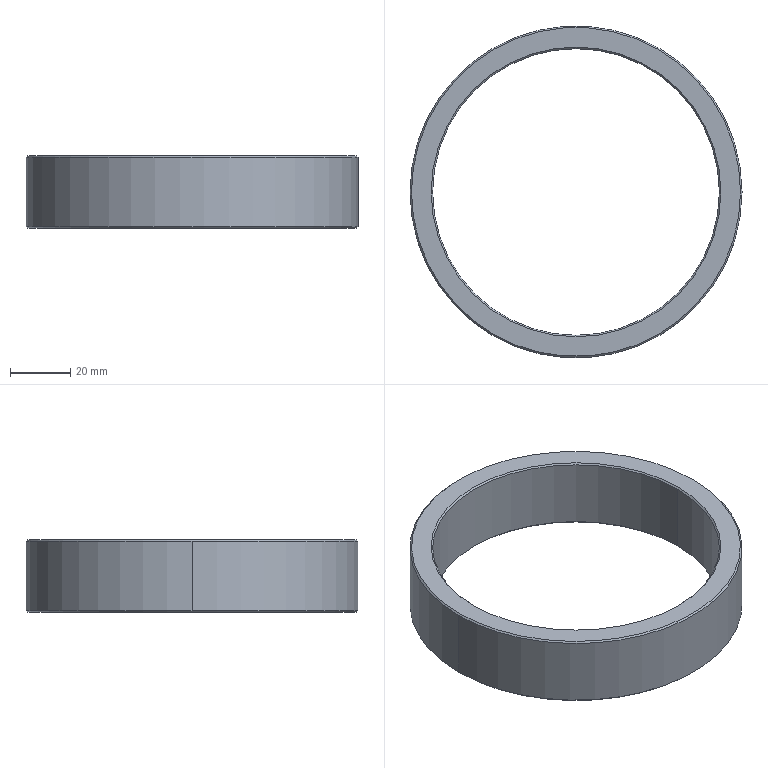Part | SolidWorks | features Chamfer 1, Extrusion 1 | 1 solid | 14 faces | box 110 x 110 x 24 mm | volume 57801 mm3 | cone 8 | cylinder 4 | plane 2 | commonest cylinder face diameters 95 x2 110 x2
STEP:
#1=CARTESIAN_POINT('',(54.5,0.,24.));
#2=VERTEX_POINT('',#1);
#3=CARTESIAN_POINT('',(-54.5,0.,24.));
#4=VERTEX_POINT('',#3);
#5=CARTESIAN_POINT('',(0.,0.,24.));
#6=DIRECTION('',(0.,0.,1.));
#7=DIRECTION('',(1.,0.,0.));
#8=AXIS2_PLACEMENT_3D('',#5,#6,#7);
#9=CIRCLE('',#8,54.5);
#10=EDGE_CURVE('',#2,#4,#9,.T.);
#11=ORIENTED_EDGE('',*,*,#10,.F.);
#12=CARTESIAN_POINT('',(55.,0.,23.5));
#13=VERTEX_POINT('',#12);
#14=CARTESIAN_POINT('',(54.5,0.,24.));
#15=DIRECTION('',(0.7071,0.,-0.7071));
#16=VECTOR('',#15,1000.);
#17=LINE('',#14,#16);
#18=EDGE_CURVE('',#2,#13,#17,.T.);
#19=ORIENTED_EDGE('',*,*,#18,.T.);
#20=CARTESIAN_POINT('',(-55.,0.,23.5));
#21=VERTEX_POINT('',#20);
#22=CARTESIAN_POINT('',(0.,0.,23.5));
#23=DIRECTION('',(0.,0.,-1.));
#24=DIRECTION('',(1.,0.,0.));
#25=AXIS2_PLACEMENT_3D('',#22,#23,#24);
#26=CIRCLE('',#25,55.);
#27=EDGE_CURVE('',#21,#13,#26,.T.);
#28=ORIENTED_EDGE('',*,*,#27,.F.);
#29=CARTESIAN_POINT('',(-54.5,0.,24.));
#30=DIRECTION('',(-0.7071,0.,-0.7071));
#31=VECTOR('',#30,1000.);
#32=LINE('',#29,#31);
#33=EDGE_CURVE('',#4,#21,#32,.T.);
#34=ORIENTED_EDGE('',*,*,#33,.F.);
#35=EDGE_LOOP('',(#11,#19,#28,#34));
#36=FACE_OUTER_BOUND('',#35,.T.);
#37=CARTESIAN_POINT('',(0.,0.,24.));
#38=DIRECTION('',(0.,0.,-1.));
#39=DIRECTION('',(-1.,0.,0.));
#40=AXIS2_PLACEMENT_3D('',#37,#38,#39);
#41=CONICAL_SURFACE('',#40,54.5,0.7854);
#42=ADVANCED_FACE('',(#36),#41,.T.);
#43=CARTESIAN_POINT('',(-47.5,0.,23.5));
#44=VERTEX_POINT('',#43);
#45=CARTESIAN_POINT('',(47.5,0.,23.5));
#46=VERTEX_POINT('',#45);
#47=CARTESIAN_POINT('',(0.,0.,23.5));
#48=DIRECTION('',(0.,0.,1.));
#49=DIRECTION('',(1.,0.,0.));
#50=AXIS2_PLACEMENT_3D('',#47,#48,#49);
#51=CIRCLE('',#50,47.5);
#52=EDGE_CURVE('',#44,#46,#51,.T.);
#53=ORIENTED_EDGE('',*,*,#52,.F.);
#54=CARTESIAN_POINT('',(-48.,0.,24.));
#55=VERTEX_POINT('',#54);
#56=CARTESIAN_POINT('',(-47.5,0.,23.5));
#57=DIRECTION('',(-0.7071,0.,0.7071));
#58=VECTOR('',#57,1000.);
#59=LINE('',#56,#58);
#60=EDGE_CURVE('',#44,#55,#59,.T.);
#61=ORIENTED_EDGE('',*,*,#60,.T.);
#62=CARTESIAN_POINT('',(48.,0.,24.));
#63=VERTEX_POINT('',#62);
#64=CARTESIAN_POINT('',(0.,0.,24.));
#65=DIRECTION('',(0.,0.,-1.));
#66=DIRECTION('',(1.,0.,0.));
#67=AXIS2_PLACEMENT_3D('',#64,#65,#66);
#68=CIRCLE('',#67,48.);
#69=EDGE_CURVE('',#63,#55,#68,.T.);
#70=ORIENTED_EDGE('',*,*,#69,.F.);
#71=CARTESIAN_POINT('',(47.5,0.,23.5));
#72=DIRECTION('',(0.7071,0.,0.7071));
#73=VECTOR('',#72,1000.);
#74=LINE('',#71,#73);
#75=EDGE_CURVE('',#46,#63,#74,.T.);
#76=ORIENTED_EDGE('',*,*,#75,.F.);
#77=EDGE_LOOP('',(#53,#61,#70,#76));
#78=FACE_OUTER_BOUND('',#77,.T.);
#79=CARTESIAN_POINT('',(0.,0.,23.5));
#80=DIRECTION('',(0.,0.,1.));
#81=DIRECTION('',(1.,0.,0.));
#82=AXIS2_PLACEMENT_3D('',#79,#80,#81);
#83=CONICAL_SURFACE('',#82,47.5,0.7854);
#84=ADVANCED_FACE('',(#78),#83,.F.);
#85=CARTESIAN_POINT('',(-54.5,0.,0.));
#86=VERTEX_POINT('',#85);
#87=CARTESIAN_POINT('',(54.5,0.,0.));
#88=VERTEX_POINT('',#87);
#89=CARTESIAN_POINT('',(0.,0.,0.));
#90=DIRECTION('',(0.,0.,-1.));
#91=DIRECTION('',(1.,0.,0.));
#92=AXIS2_PLACEMENT_3D('',#89,#90,#91);
#93=CIRCLE('',#92,54.5);
#94=EDGE_CURVE('',#86,#88,#93,.T.);
#95=ORIENTED_EDGE('',*,*,#94,.F.);
#96=CARTESIAN_POINT('',(-55.,0.,0.5));
#97=VERTEX_POINT('',#96);
#98=CARTESIAN_POINT('',(-55.,0.,0.5));
#99=DIRECTION('',(-0.7071,0.,0.7071));
#100=VECTOR('',#99,1000.);
#101=LINE('',#98,#100);
#102=EDGE_CURVE('',#86,#97,#101,.T.);
#103=ORIENTED_EDGE('',*,*,#102,.T.);
#104=CARTESIAN_POINT('',(55.,0.,0.5));
#105=VERTEX_POINT('',#104);
#106=CARTESIAN_POINT('',(0.,0.,0.5));
#107=DIRECTION('',(0.,0.,1.));
#108=DIRECTION('',(1.,0.,0.));
#109=AXIS2_PLACEMENT_3D('',#106,#107,#108);
#110=CIRCLE('',#109,55.);
#111=EDGE_CURVE('',#105,#97,#110,.T.);
#112=ORIENTED_EDGE('',*,*,#111,.F.);
#113=CARTESIAN_POINT('',(55.,0.,0.5));
#114=DIRECTION('',(0.7071,0.,0.7071));
#115=VECTOR('',#114,1000.);
#116=LINE('',#113,#115);
#117=EDGE_CURVE('',#88,#105,#116,.T.);
#118=ORIENTED_EDGE('',*,*,#117,.F.);
#119=EDGE_LOOP('',(#95,#103,#112,#118));
#120=FACE_OUTER_BOUND('',#119,.T.);
#121=CARTESIAN_POINT('',(0.,0.,0.5));
#122=DIRECTION('',(0.,0.,1.));
#123=DIRECTION('',(1.,0.,0.));
#124=AXIS2_PLACEMENT_3D('',#121,#122,#123);
#125=CONICAL_SURFACE('',#124,55.,0.7854);
#126=ADVANCED_FACE('',(#120),#125,.T.);
#127=CARTESIAN_POINT('',(47.5,0.,0.5));
#128=VERTEX_POINT('',#127);
#129=CARTESIAN_POINT('',(-47.5,0.,0.5));
#130=VERTEX_POINT('',#129);
#131=CARTESIAN_POINT('',(0.,0.,0.5));
#132=DIRECTION('',(0.,0.,-1.));
#133=DIRECTION('',(1.,0.,0.));
#134=AXIS2_PLACEMENT_3D('',#131,#132,#133);
#135=CIRCLE('',#134,47.5);
#136=EDGE_CURVE('',#128,#130,#135,.T.);
#137=ORIENTED_EDGE('',*,*,#136,.F.);
#138=CARTESIAN_POINT('',(48.,0.,0.));
#139=VERTEX_POINT('',#138);
#140=CARTESIAN_POINT('',(48.,0.,0.));
#141=DIRECTION('',(0.7071,0.,-0.7071));
#142=VECTOR('',#141,1000.);
#143=LINE('',#140,#142);
#144=EDGE_CURVE('',#128,#139,#143,.T.);
#145=ORIENTED_EDGE('',*,*,#144,.T.);
#146=CARTESIAN_POINT('',(-48.,0.,0.));
#147=VERTEX_POINT('',#146);
#148=CARTESIAN_POINT('',(0.,0.,0.));
#149=DIRECTION('',(0.,0.,1.));
#150=DIRECTION('',(1.,0.,0.));
#151=AXIS2_PLACEMENT_3D('',#148,#149,#150);
#152=CIRCLE('',#151,48.);
#153=EDGE_CURVE('',#147,#139,#152,.T.);
#154=ORIENTED_EDGE('',*,*,#153,.F.);
#155=CARTESIAN_POINT('',(-48.,0.,0.));
#156=DIRECTION('',(-0.7071,0.,-0.7071));
#157=VECTOR('',#156,1000.);
#158=LINE('',#155,#157);
#159=EDGE_CURVE('',#130,#147,#158,.T.);
#160=ORIENTED_EDGE('',*,*,#159,.F.);
#161=EDGE_LOOP('',(#137,#145,#154,#160));
#162=FACE_OUTER_BOUND('',#161,.T.);
#163=CARTESIAN_POINT('',(0.,0.,0.));
#164=DIRECTION('',(0.,0.,-1.));
#165=DIRECTION('',(-1.,0.,0.));
#166=AXIS2_PLACEMENT_3D('',#163,#164,#165);
#167=CONICAL_SURFACE('',#166,48.,0.7854);
#168=ADVANCED_FACE('',(#162),#167,.F.);
#169=ORIENTED_EDGE('',*,*,#52,.T.);
#170=CARTESIAN_POINT('',(47.5,0.,24.));
#171=DIRECTION('',(0.,0.,-1.));
#172=VECTOR('',#171,1000.);
#173=LINE('',#170,#172);
#174=EDGE_CURVE('',#46,#128,#173,.T.);
#175=ORIENTED_EDGE('',*,*,#174,.T.);
#176=ORIENTED_EDGE('',*,*,#136,.T.);
#177=CARTESIAN_POINT('',(-47.5,0.,24.));
#178=DIRECTION('',(0.,0.,-1.));
#179=VECTOR('',#178,1000.);
#180=LINE('',#177,#179);
#181=EDGE_CURVE('',#44,#130,#180,.T.);
#182=ORIENTED_EDGE('',*,*,#181,.F.);
#183=EDGE_LOOP('',(#169,#175,#176,#182));
#184=FACE_OUTER_BOUND('',#183,.T.);
#185=CARTESIAN_POINT('',(0.,0.,24.));
#186=DIRECTION('',(0.,0.,-1.));
#187=DIRECTION('',(-1.,0.,0.));
#188=AXIS2_PLACEMENT_3D('',#185,#186,#187);
#189=CYLINDRICAL_SURFACE('',#188,47.5);
#190=ADVANCED_FACE('',(#184),#189,.F.);
#191=ORIENTED_EDGE('',*,*,#27,.T.);
#192=CARTESIAN_POINT('',(55.,0.,24.));
#193=DIRECTION('',(0.,0.,-1.));
#194=VECTOR('',#193,1000.);
#195=LINE('',#192,#194);
#196=EDGE_CURVE('',#13,#105,#195,.T.);
#197=ORIENTED_EDGE('',*,*,#196,.T.);
#198=ORIENTED_EDGE('',*,*,#111,.T.);
#199=CARTESIAN_POINT('',(-55.,0.,24.));
#200=DIRECTION('',(0.,0.,-1.));
#201=VECTOR('',#200,1000.);
#202=LINE('',#199,#201);
#203=EDGE_CURVE('',#21,#97,#202,.T.);
#204=ORIENTED_EDGE('',*,*,#203,.F.);
#205=EDGE_LOOP('',(#191,#197,#198,#204));
#206=FACE_OUTER_BOUND('',#205,.T.);
#207=CARTESIAN_POINT('',(0.,0.,24.));
#208=DIRECTION('',(0.,0.,-1.));
#209=DIRECTION('',(-1.,0.,0.));
#210=AXIS2_PLACEMENT_3D('',#207,#208,#209);
#211=CYLINDRICAL_SURFACE('',#210,55.);
#212=ADVANCED_FACE('',(#206),#211,.T.);
#213=ORIENTED_EDGE('',*,*,#69,.T.);
#214=CARTESIAN_POINT('',(0.,0.,24.));
#215=DIRECTION('',(0.,0.,-1.));
#216=DIRECTION('',(1.,0.,0.));
#217=AXIS2_PLACEMENT_3D('',#214,#215,#216);
#218=CIRCLE('',#217,48.);
#219=EDGE_CURVE('',#55,#63,#218,.T.);
#220=ORIENTED_EDGE('',*,*,#219,.T.);
#221=EDGE_LOOP('',(#213,#220));
#222=FACE_BOUND('',#221,.T.);
#223=CARTESIAN_POINT('',(0.,0.,24.));
#224=DIRECTION('',(0.,0.,1.));
#225=DIRECTION('',(1.,0.,0.));
#226=AXIS2_PLACEMENT_3D('',#223,#224,#225);
#227=CIRCLE('',#226,54.5);
#228=EDGE_CURVE('',#4,#2,#227,.T.);
#229=ORIENTED_EDGE('',*,*,#228,.T.);
#230=ORIENTED_EDGE('',*,*,#10,.T.);
#231=EDGE_LOOP('',(#229,#230));
#232=FACE_OUTER_BOUND('',#231,.T.);
#233=CARTESIAN_POINT('',(0.,0.,24.));
#234=DIRECTION('',(0.,0.,1.));
#235=DIRECTION('',(1.,0.,0.));
#236=AXIS2_PLACEMENT_3D('',#233,#234,#235);
#237=PLANE('',#236);
#238=ADVANCED_FACE('',(#222,#232),#237,.T.);
#239=ORIENTED_EDGE('',*,*,#153,.T.);
#240=CARTESIAN_POINT('',(0.,0.,0.));
#241=DIRECTION('',(0.,0.,1.));
#242=DIRECTION('',(1.,0.,0.));
#243=AXIS2_PLACEMENT_3D('',#240,#241,#242);
#244=CIRCLE('',#243,48.);
#245=EDGE_CURVE('',#139,#147,#244,.T.);
#246=ORIENTED_EDGE('',*,*,#245,.T.);
#247=EDGE_LOOP('',(#239,#246));
#248=FACE_BOUND('',#247,.T.);
#249=CARTESIAN_POINT('',(0.,0.,0.));
#250=DIRECTION('',(0.,0.,-1.));
#251=DIRECTION('',(1.,0.,0.));
#252=AXIS2_PLACEMENT_3D('',#249,#250,#251);
#253=CIRCLE('',#252,54.5);
#254=EDGE_CURVE('',#88,#86,#253,.T.);
#255=ORIENTED_EDGE('',*,*,#254,.T.);
#256=ORIENTED_EDGE('',*,*,#94,.T.);
#257=EDGE_LOOP('',(#255,#256));
#258=FACE_OUTER_BOUND('',#257,.T.);
#259=CARTESIAN_POINT('',(0.,0.,0.));
#260=DIRECTION('',(0.,0.,1.));
#261=DIRECTION('',(1.,0.,0.));
#262=AXIS2_PLACEMENT_3D('',#259,#260,#261);
#263=PLANE('',#262);
#264=ADVANCED_FACE('',(#248,#258),#263,.F.);
#265=ORIENTED_EDGE('',*,*,#196,.F.);
#266=CARTESIAN_POINT('',(0.,0.,23.5));
#267=DIRECTION('',(0.,0.,-1.));
#268=DIRECTION('',(1.,0.,0.));
#269=AXIS2_PLACEMENT_3D('',#266,#267,#268);
#270=CIRCLE('',#269,55.);
#271=EDGE_CURVE('',#13,#21,#270,.T.);
#272=ORIENTED_EDGE('',*,*,#271,.T.);
#273=ORIENTED_EDGE('',*,*,#203,.T.);
#274=CARTESIAN_POINT('',(0.,0.,0.5));
#275=DIRECTION('',(0.,0.,1.));
#276=DIRECTION('',(1.,0.,0.));
#277=AXIS2_PLACEMENT_3D('',#274,#275,#276);
#278=CIRCLE('',#277,55.);
#279=EDGE_CURVE('',#97,#105,#278,.T.);
#280=ORIENTED_EDGE('',*,*,#279,.T.);
#281=EDGE_LOOP('',(#265,#272,#273,#280));
#282=FACE_OUTER_BOUND('',#281,.T.);
#283=CARTESIAN_POINT('',(0.,0.,24.));
#284=DIRECTION('',(0.,0.,-1.));
#285=DIRECTION('',(-1.,0.,0.));
#286=AXIS2_PLACEMENT_3D('',#283,#284,#285);
#287=CYLINDRICAL_SURFACE('',#286,55.);
#288=ADVANCED_FACE('',(#282),#287,.T.);
#289=ORIENTED_EDGE('',*,*,#174,.F.);
#290=CARTESIAN_POINT('',(0.,0.,23.5));
#291=DIRECTION('',(0.,0.,1.));
#292=DIRECTION('',(1.,0.,0.));
#293=AXIS2_PLACEMENT_3D('',#290,#291,#292);
#294=CIRCLE('',#293,47.5);
#295=EDGE_CURVE('',#46,#44,#294,.T.);
#296=ORIENTED_EDGE('',*,*,#295,.T.);
#297=ORIENTED_EDGE('',*,*,#181,.T.);
#298=CARTESIAN_POINT('',(0.,0.,0.5));
#299=DIRECTION('',(0.,0.,-1.));
#300=DIRECTION('',(1.,0.,0.));
#301=AXIS2_PLACEMENT_3D('',#298,#299,#300);
#302=CIRCLE('',#301,47.5);
#303=EDGE_CURVE('',#130,#128,#302,.T.);
#304=ORIENTED_EDGE('',*,*,#303,.T.);
#305=EDGE_LOOP('',(#289,#296,#297,#304));
#306=FACE_OUTER_BOUND('',#305,.T.);
#307=CARTESIAN_POINT('',(0.,0.,24.));
#308=DIRECTION('',(0.,0.,-1.));
#309=DIRECTION('',(-1.,0.,0.));
#310=AXIS2_PLACEMENT_3D('',#307,#308,#309);
#311=CYLINDRICAL_SURFACE('',#310,47.5);
#312=ADVANCED_FACE('',(#306),#311,.F.);
#313=ORIENTED_EDGE('',*,*,#144,.F.);
#314=ORIENTED_EDGE('',*,*,#303,.F.);
#315=ORIENTED_EDGE('',*,*,#159,.T.);
#316=ORIENTED_EDGE('',*,*,#245,.F.);
#317=EDGE_LOOP('',(#313,#314,#315,#316));
#318=FACE_OUTER_BOUND('',#317,.T.);
#319=CARTESIAN_POINT('',(0.,0.,0.));
#320=DIRECTION('',(0.,0.,-1.));
#321=DIRECTION('',(-1.,0.,0.));
#322=AXIS2_PLACEMENT_3D('',#319,#320,#321);
#323=CONICAL_SURFACE('',#322,48.,0.7854);
#324=ADVANCED_FACE('',(#318),#323,.F.);
#325=ORIENTED_EDGE('',*,*,#102,.F.);
#326=ORIENTED_EDGE('',*,*,#254,.F.);
#327=ORIENTED_EDGE('',*,*,#117,.T.);
#328=ORIENTED_EDGE('',*,*,#279,.F.);
#329=EDGE_LOOP('',(#325,#326,#327,#328));
#330=FACE_OUTER_BOUND('',#329,.T.);
#331=CARTESIAN_POINT('',(0.,0.,0.5));
#332=DIRECTION('',(0.,0.,1.));
#333=DIRECTION('',(1.,0.,0.));
#334=AXIS2_PLACEMENT_3D('',#331,#332,#333);
#335=CONICAL_SURFACE('',#334,55.,0.7854);
#336=ADVANCED_FACE('',(#330),#335,.T.);
#337=ORIENTED_EDGE('',*,*,#60,.F.);
#338=ORIENTED_EDGE('',*,*,#295,.F.);
#339=ORIENTED_EDGE('',*,*,#75,.T.);
#340=ORIENTED_EDGE('',*,*,#219,.F.);
#341=EDGE_LOOP('',(#337,#338,#339,#340));
#342=FACE_OUTER_BOUND('',#341,.T.);
#343=CARTESIAN_POINT('',(0.,0.,23.5));
#344=DIRECTION('',(0.,0.,1.));
#345=DIRECTION('',(1.,0.,0.));
#346=AXIS2_PLACEMENT_3D('',#343,#344,#345);
#347=CONICAL_SURFACE('',#346,47.5,0.7854);
#348=ADVANCED_FACE('',(#342),#347,.F.);
#349=ORIENTED_EDGE('',*,*,#18,.F.);
#350=ORIENTED_EDGE('',*,*,#228,.F.);
#351=ORIENTED_EDGE('',*,*,#33,.T.);
#352=ORIENTED_EDGE('',*,*,#271,.F.);
#353=EDGE_LOOP('',(#349,#350,#351,#352));
#354=FACE_OUTER_BOUND('',#353,.T.);
#355=CARTESIAN_POINT('',(0.,0.,24.));
#356=DIRECTION('',(0.,0.,-1.));
#357=DIRECTION('',(-1.,0.,0.));
#358=AXIS2_PLACEMENT_3D('',#355,#356,#357);
#359=CONICAL_SURFACE('',#358,54.5,0.7854);
#360=ADVANCED_FACE('',(#354),#359,.T.);
#361=CLOSED_SHELL('',(#42,#84,#126,#168,#190,#212,#238,#264,#288,#312,#324,#336,#348,#360));
#362=MANIFOLD_SOLID_BREP('',#361);
#363=CARTESIAN_POINT('',(0.,0.,0.));
#364=DIRECTION('',(0.,0.,1.));
#365=DIRECTION('',(1.,0.,0.));
#366=AXIS2_PLACEMENT_3D('',#363,#364,#365);
#367=(LENGTH_UNIT()NAMED_UNIT(*)SI_UNIT(.MILLI.,.METRE.));
#368=UNCERTAINTY_MEASURE_WITH_UNIT(LENGTH_MEASURE(0.00001),#367,'','');
#369=(NAMED_UNIT(*)PLANE_ANGLE_UNIT()SI_UNIT($,.RADIAN.));
#370=(NAMED_UNIT(*)SI_UNIT($,.STERADIAN.)SOLID_ANGLE_UNIT());
#371=(GEOMETRIC_REPRESENTATION_CONTEXT(3)GLOBAL_UNCERTAINTY_ASSIGNED_CONTEXT((#368))GLOBAL_UNIT_ASSIGNED_CONTEXT((#367,#369,#370))REPRESENTATION_CONTEXT('',''));
#372=ADVANCED_BREP_SHAPE_REPRESENTATION('',(#362,#366),#371);